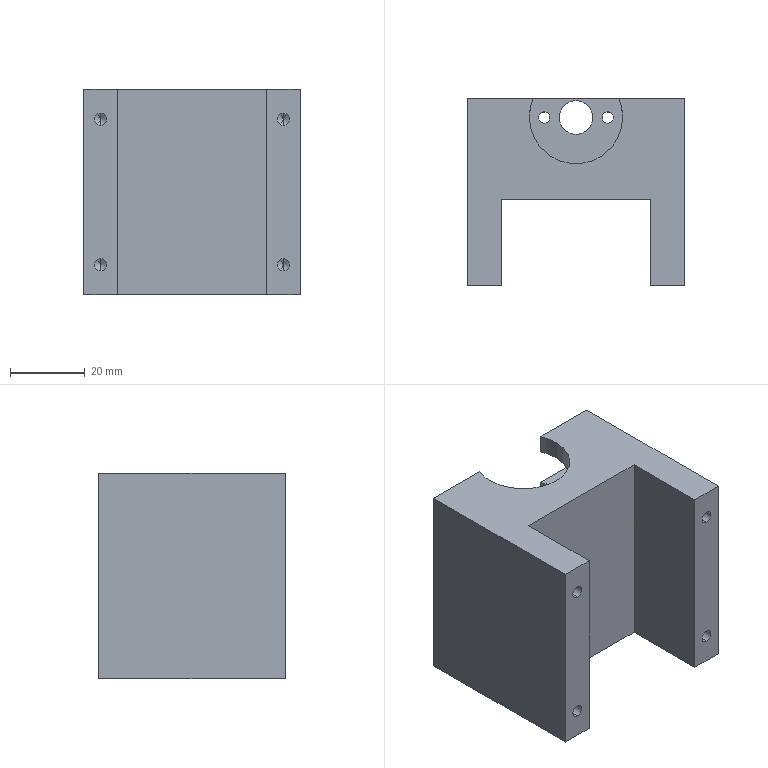Part | SolidWorks | features ICE 4, Extrusion 1, HoleWzd 1 | 1 solid | 60 faces | box 58 x 50 x 55 mm | volume 71255 mm3 | cylinder 26 | plane 26 | cone 8 | commonest cylinder face diameters 25 x12 3.3 x8 3 x4 9 x2